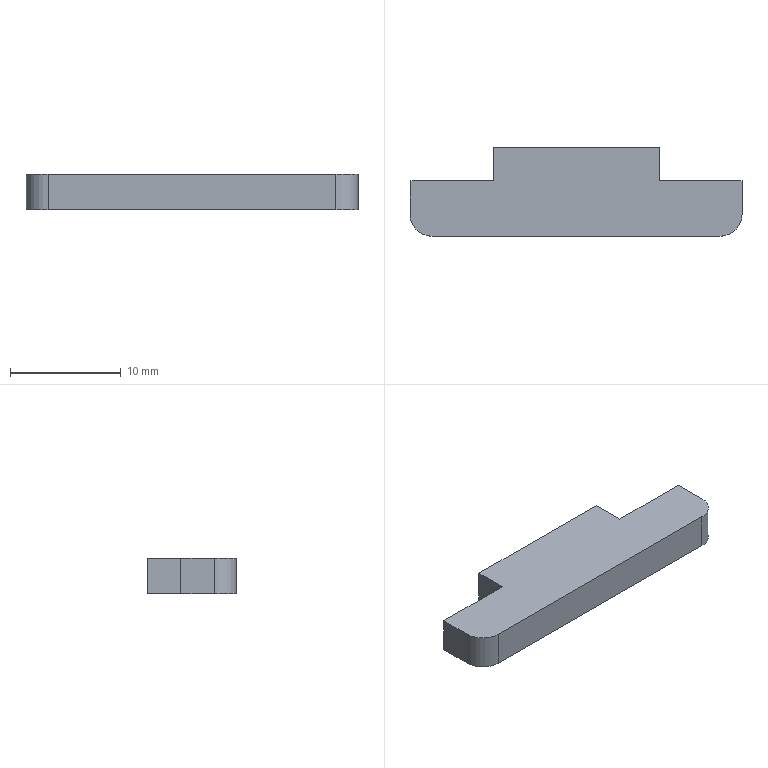Part | SolidWorks | features FlatPattern 1, SMBaseFlange 1, SheetMetal 1 | 1 solid | 12 faces | box 30 x 8 x 3.2 mm | volume 618.506 mm3 | plane 10 | cylinder 2 | commonest cylinder face diameters 4 x2
STEP:
#1=CARTESIAN_POINT('',(-119.188,177.146,0.));
#2=VERTEX_POINT('',#1);
#3=CARTESIAN_POINT('',(-119.188,180.146,0.));
#4=VERTEX_POINT('',#3);
#5=CARTESIAN_POINT('',(-119.188,177.146,0.));
#6=DIRECTION('',(0.,1.,0.));
#7=VECTOR('',#6,1000.);
#8=LINE('',#5,#7);
#9=EDGE_CURVE('',#2,#4,#8,.T.);
#10=ORIENTED_EDGE('',*,*,#9,.F.);
#11=CARTESIAN_POINT('',(-119.188,177.146,-3.2));
#12=VERTEX_POINT('',#11);
#13=CARTESIAN_POINT('',(-119.188,177.146,-3.2));
#14=DIRECTION('',(0.,0.,1.));
#15=VECTOR('',#14,1000.);
#16=LINE('',#13,#15);
#17=EDGE_CURVE('',#12,#2,#16,.T.);
#18=ORIENTED_EDGE('',*,*,#17,.F.);
#19=CARTESIAN_POINT('',(-119.188,180.146,-3.2));
#20=VERTEX_POINT('',#19);
#21=CARTESIAN_POINT('',(-119.188,177.146,-3.2));
#22=DIRECTION('',(0.,1.,0.));
#23=VECTOR('',#22,1000.);
#24=LINE('',#21,#23);
#25=EDGE_CURVE('',#12,#20,#24,.T.);
#26=ORIENTED_EDGE('',*,*,#25,.T.);
#27=CARTESIAN_POINT('',(-119.188,180.146,-3.2));
#28=DIRECTION('',(0.,0.,1.));
#29=VECTOR('',#28,1000.);
#30=LINE('',#27,#29);
#31=EDGE_CURVE('',#20,#4,#30,.T.);
#32=ORIENTED_EDGE('',*,*,#31,.T.);
#33=EDGE_LOOP('',(#10,#18,#26,#32));
#34=FACE_OUTER_BOUND('',#33,.T.);
#35=CARTESIAN_POINT('',(-119.188,177.146,-3.2));
#36=DIRECTION('',(1.,0.,0.));
#37=DIRECTION('',(0.,0.,-1.));
#38=AXIS2_PLACEMENT_3D('',#35,#36,#37);
#39=PLANE('',#38);
#40=ADVANCED_FACE('',(#34),#39,.T.);
#41=CARTESIAN_POINT('',(-121.188,175.146,0.));
#42=VERTEX_POINT('',#41);
#43=CARTESIAN_POINT('',(-121.188,177.146,0.));
#44=DIRECTION('',(0.,0.,1.));
#45=DIRECTION('',(1.,0.,0.));
#46=AXIS2_PLACEMENT_3D('',#43,#44,#45);
#47=CIRCLE('',#46,2.);
#48=EDGE_CURVE('',#42,#2,#47,.T.);
#49=ORIENTED_EDGE('',*,*,#48,.F.);
#50=CARTESIAN_POINT('',(-121.188,175.146,-3.2));
#51=VERTEX_POINT('',#50);
#52=CARTESIAN_POINT('',(-121.188,175.146,-3.2));
#53=DIRECTION('',(0.,0.,1.));
#54=VECTOR('',#53,1000.);
#55=LINE('',#52,#54);
#56=EDGE_CURVE('',#51,#42,#55,.T.);
#57=ORIENTED_EDGE('',*,*,#56,.F.);
#58=CARTESIAN_POINT('',(-121.188,177.146,-3.2));
#59=DIRECTION('',(0.,0.,1.));
#60=DIRECTION('',(1.,0.,0.));
#61=AXIS2_PLACEMENT_3D('',#58,#59,#60);
#62=CIRCLE('',#61,2.);
#63=EDGE_CURVE('',#51,#12,#62,.T.);
#64=ORIENTED_EDGE('',*,*,#63,.T.);
#65=ORIENTED_EDGE('',*,*,#17,.T.);
#66=EDGE_LOOP('',(#49,#57,#64,#65));
#67=FACE_OUTER_BOUND('',#66,.T.);
#68=CARTESIAN_POINT('',(-121.188,177.146,-3.2));
#69=DIRECTION('',(0.,0.,1.));
#70=DIRECTION('',(1.,0.,0.));
#71=AXIS2_PLACEMENT_3D('',#68,#69,#70);
#72=CYLINDRICAL_SURFACE('',#71,2.);
#73=ADVANCED_FACE('',(#67),#72,.T.);
#74=CARTESIAN_POINT('',(-147.188,175.146,0.));
#75=VERTEX_POINT('',#74);
#76=CARTESIAN_POINT('',(-147.188,175.146,0.));
#77=DIRECTION('',(1.,0.,0.));
#78=VECTOR('',#77,1000.);
#79=LINE('',#76,#78);
#80=EDGE_CURVE('',#75,#42,#79,.T.);
#81=ORIENTED_EDGE('',*,*,#80,.F.);
#82=CARTESIAN_POINT('',(-147.188,175.146,-3.2));
#83=VERTEX_POINT('',#82);
#84=CARTESIAN_POINT('',(-147.188,175.146,-3.2));
#85=DIRECTION('',(0.,0.,1.));
#86=VECTOR('',#85,1000.);
#87=LINE('',#84,#86);
#88=EDGE_CURVE('',#83,#75,#87,.T.);
#89=ORIENTED_EDGE('',*,*,#88,.F.);
#90=CARTESIAN_POINT('',(-147.188,175.146,-3.2));
#91=DIRECTION('',(1.,0.,0.));
#92=VECTOR('',#91,1000.);
#93=LINE('',#90,#92);
#94=EDGE_CURVE('',#83,#51,#93,.T.);
#95=ORIENTED_EDGE('',*,*,#94,.T.);
#96=ORIENTED_EDGE('',*,*,#56,.T.);
#97=EDGE_LOOP('',(#81,#89,#95,#96));
#98=FACE_OUTER_BOUND('',#97,.T.);
#99=CARTESIAN_POINT('',(-147.188,175.146,-3.2));
#100=DIRECTION('',(0.,-1.,0.));
#101=DIRECTION('',(0.,0.,-1.));
#102=AXIS2_PLACEMENT_3D('',#99,#100,#101);
#103=PLANE('',#102);
#104=ADVANCED_FACE('',(#98),#103,.T.);
#105=CARTESIAN_POINT('',(-149.188,177.146,0.));
#106=VERTEX_POINT('',#105);
#107=CARTESIAN_POINT('',(-147.188,177.146,0.));
#108=DIRECTION('',(0.,0.,1.));
#109=DIRECTION('',(1.,0.,0.));
#110=AXIS2_PLACEMENT_3D('',#107,#108,#109);
#111=CIRCLE('',#110,2.);
#112=EDGE_CURVE('',#106,#75,#111,.T.);
#113=ORIENTED_EDGE('',*,*,#112,.F.);
#114=CARTESIAN_POINT('',(-149.188,177.146,-3.2));
#115=VERTEX_POINT('',#114);
#116=CARTESIAN_POINT('',(-149.188,177.146,-3.2));
#117=DIRECTION('',(0.,0.,1.));
#118=VECTOR('',#117,1000.);
#119=LINE('',#116,#118);
#120=EDGE_CURVE('',#115,#106,#119,.T.);
#121=ORIENTED_EDGE('',*,*,#120,.F.);
#122=CARTESIAN_POINT('',(-147.188,177.146,-3.2));
#123=DIRECTION('',(0.,0.,1.));
#124=DIRECTION('',(1.,0.,0.));
#125=AXIS2_PLACEMENT_3D('',#122,#123,#124);
#126=CIRCLE('',#125,2.);
#127=EDGE_CURVE('',#115,#83,#126,.T.);
#128=ORIENTED_EDGE('',*,*,#127,.T.);
#129=ORIENTED_EDGE('',*,*,#88,.T.);
#130=EDGE_LOOP('',(#113,#121,#128,#129));
#131=FACE_OUTER_BOUND('',#130,.T.);
#132=CARTESIAN_POINT('',(-147.188,177.146,-3.2));
#133=DIRECTION('',(0.,0.,1.));
#134=DIRECTION('',(1.,0.,0.));
#135=AXIS2_PLACEMENT_3D('',#132,#133,#134);
#136=CYLINDRICAL_SURFACE('',#135,2.);
#137=ADVANCED_FACE('',(#131),#136,.T.);
#138=CARTESIAN_POINT('',(-149.188,180.146,0.));
#139=VERTEX_POINT('',#138);
#140=CARTESIAN_POINT('',(-149.188,180.146,0.));
#141=DIRECTION('',(0.,-1.,0.));
#142=VECTOR('',#141,1000.);
#143=LINE('',#140,#142);
#144=EDGE_CURVE('',#139,#106,#143,.T.);
#145=ORIENTED_EDGE('',*,*,#144,.F.);
#146=CARTESIAN_POINT('',(-149.188,180.146,-3.2));
#147=VERTEX_POINT('',#146);
#148=CARTESIAN_POINT('',(-149.188,180.146,-3.2));
#149=DIRECTION('',(0.,0.,1.));
#150=VECTOR('',#149,1000.);
#151=LINE('',#148,#150);
#152=EDGE_CURVE('',#147,#139,#151,.T.);
#153=ORIENTED_EDGE('',*,*,#152,.F.);
#154=CARTESIAN_POINT('',(-149.188,180.146,-3.2));
#155=DIRECTION('',(0.,-1.,0.));
#156=VECTOR('',#155,1000.);
#157=LINE('',#154,#156);
#158=EDGE_CURVE('',#147,#115,#157,.T.);
#159=ORIENTED_EDGE('',*,*,#158,.T.);
#160=ORIENTED_EDGE('',*,*,#120,.T.);
#161=EDGE_LOOP('',(#145,#153,#159,#160));
#162=FACE_OUTER_BOUND('',#161,.T.);
#163=CARTESIAN_POINT('',(-149.188,180.146,-3.2));
#164=DIRECTION('',(-1.,0.,0.));
#165=DIRECTION('',(0.,0.,1.));
#166=AXIS2_PLACEMENT_3D('',#163,#164,#165);
#167=PLANE('',#166);
#168=ADVANCED_FACE('',(#162),#167,.T.);
#169=CARTESIAN_POINT('',(-141.688,180.146,0.));
#170=VERTEX_POINT('',#169);
#171=CARTESIAN_POINT('',(-141.688,180.146,0.));
#172=DIRECTION('',(-1.,0.,0.));
#173=VECTOR('',#172,1000.);
#174=LINE('',#171,#173);
#175=EDGE_CURVE('',#170,#139,#174,.T.);
#176=ORIENTED_EDGE('',*,*,#175,.F.);
#177=CARTESIAN_POINT('',(-141.688,180.146,-3.2));
#178=VERTEX_POINT('',#177);
#179=CARTESIAN_POINT('',(-141.688,180.146,-3.2));
#180=DIRECTION('',(0.,0.,1.));
#181=VECTOR('',#180,1000.);
#182=LINE('',#179,#181);
#183=EDGE_CURVE('',#178,#170,#182,.T.);
#184=ORIENTED_EDGE('',*,*,#183,.F.);
#185=CARTESIAN_POINT('',(-141.688,180.146,-3.2));
#186=DIRECTION('',(-1.,0.,0.));
#187=VECTOR('',#186,1000.);
#188=LINE('',#185,#187);
#189=EDGE_CURVE('',#178,#147,#188,.T.);
#190=ORIENTED_EDGE('',*,*,#189,.T.);
#191=ORIENTED_EDGE('',*,*,#152,.T.);
#192=EDGE_LOOP('',(#176,#184,#190,#191));
#193=FACE_OUTER_BOUND('',#192,.T.);
#194=CARTESIAN_POINT('',(-141.688,180.146,-3.2));
#195=DIRECTION('',(0.,1.,0.));
#196=DIRECTION('',(0.,0.,1.));
#197=AXIS2_PLACEMENT_3D('',#194,#195,#196);
#198=PLANE('',#197);
#199=ADVANCED_FACE('',(#193),#198,.T.);
#200=CARTESIAN_POINT('',(-141.688,183.146,0.));
#201=VERTEX_POINT('',#200);
#202=CARTESIAN_POINT('',(-141.688,183.146,0.));
#203=DIRECTION('',(0.,-1.,0.));
#204=VECTOR('',#203,1000.);
#205=LINE('',#202,#204);
#206=EDGE_CURVE('',#201,#170,#205,.T.);
#207=ORIENTED_EDGE('',*,*,#206,.F.);
#208=CARTESIAN_POINT('',(-141.688,183.146,-3.2));
#209=VERTEX_POINT('',#208);
#210=CARTESIAN_POINT('',(-141.688,183.146,-3.2));
#211=DIRECTION('',(0.,0.,1.));
#212=VECTOR('',#211,1000.);
#213=LINE('',#210,#212);
#214=EDGE_CURVE('',#209,#201,#213,.T.);
#215=ORIENTED_EDGE('',*,*,#214,.F.);
#216=CARTESIAN_POINT('',(-141.688,183.146,-3.2));
#217=DIRECTION('',(0.,-1.,0.));
#218=VECTOR('',#217,1000.);
#219=LINE('',#216,#218);
#220=EDGE_CURVE('',#209,#178,#219,.T.);
#221=ORIENTED_EDGE('',*,*,#220,.T.);
#222=ORIENTED_EDGE('',*,*,#183,.T.);
#223=EDGE_LOOP('',(#207,#215,#221,#222));
#224=FACE_OUTER_BOUND('',#223,.T.);
#225=CARTESIAN_POINT('',(-141.688,183.146,-3.2));
#226=DIRECTION('',(-1.,0.,0.));
#227=DIRECTION('',(0.,0.,1.));
#228=AXIS2_PLACEMENT_3D('',#225,#226,#227);
#229=PLANE('',#228);
#230=ADVANCED_FACE('',(#224),#229,.T.);
#231=CARTESIAN_POINT('',(-126.688,183.146,0.));
#232=VERTEX_POINT('',#231);
#233=CARTESIAN_POINT('',(-126.688,183.146,0.));
#234=DIRECTION('',(-1.,0.,0.));
#235=VECTOR('',#234,1000.);
#236=LINE('',#233,#235);
#237=EDGE_CURVE('',#232,#201,#236,.T.);
#238=ORIENTED_EDGE('',*,*,#237,.F.);
#239=CARTESIAN_POINT('',(-126.688,183.146,-3.2));
#240=VERTEX_POINT('',#239);
#241=CARTESIAN_POINT('',(-126.688,183.146,-3.2));
#242=DIRECTION('',(0.,0.,1.));
#243=VECTOR('',#242,1000.);
#244=LINE('',#241,#243);
#245=EDGE_CURVE('',#240,#232,#244,.T.);
#246=ORIENTED_EDGE('',*,*,#245,.F.);
#247=CARTESIAN_POINT('',(-126.688,183.146,-3.2));
#248=DIRECTION('',(-1.,0.,0.));
#249=VECTOR('',#248,1000.);
#250=LINE('',#247,#249);
#251=EDGE_CURVE('',#240,#209,#250,.T.);
#252=ORIENTED_EDGE('',*,*,#251,.T.);
#253=ORIENTED_EDGE('',*,*,#214,.T.);
#254=EDGE_LOOP('',(#238,#246,#252,#253));
#255=FACE_OUTER_BOUND('',#254,.T.);
#256=CARTESIAN_POINT('',(-126.688,183.146,-3.2));
#257=DIRECTION('',(0.,1.,0.));
#258=DIRECTION('',(0.,0.,1.));
#259=AXIS2_PLACEMENT_3D('',#256,#257,#258);
#260=PLANE('',#259);
#261=ADVANCED_FACE('',(#255),#260,.T.);
#262=CARTESIAN_POINT('',(-126.688,180.146,0.));
#263=VERTEX_POINT('',#262);
#264=CARTESIAN_POINT('',(-126.688,180.146,0.));
#265=DIRECTION('',(0.,1.,0.));
#266=VECTOR('',#265,1000.);
#267=LINE('',#264,#266);
#268=EDGE_CURVE('',#263,#232,#267,.T.);
#269=ORIENTED_EDGE('',*,*,#268,.F.);
#270=CARTESIAN_POINT('',(-126.688,180.146,-3.2));
#271=VERTEX_POINT('',#270);
#272=CARTESIAN_POINT('',(-126.688,180.146,-3.2));
#273=DIRECTION('',(0.,0.,1.));
#274=VECTOR('',#273,1000.);
#275=LINE('',#272,#274);
#276=EDGE_CURVE('',#271,#263,#275,.T.);
#277=ORIENTED_EDGE('',*,*,#276,.F.);
#278=CARTESIAN_POINT('',(-126.688,180.146,-3.2));
#279=DIRECTION('',(0.,1.,0.));
#280=VECTOR('',#279,1000.);
#281=LINE('',#278,#280);
#282=EDGE_CURVE('',#271,#240,#281,.T.);
#283=ORIENTED_EDGE('',*,*,#282,.T.);
#284=ORIENTED_EDGE('',*,*,#245,.T.);
#285=EDGE_LOOP('',(#269,#277,#283,#284));
#286=FACE_OUTER_BOUND('',#285,.T.);
#287=CARTESIAN_POINT('',(-126.688,180.146,-3.2));
#288=DIRECTION('',(1.,0.,0.));
#289=DIRECTION('',(0.,0.,-1.));
#290=AXIS2_PLACEMENT_3D('',#287,#288,#289);
#291=PLANE('',#290);
#292=ADVANCED_FACE('',(#286),#291,.T.);
#293=CARTESIAN_POINT('',(-119.188,180.146,0.));
#294=DIRECTION('',(-1.,0.,0.));
#295=VECTOR('',#294,1000.);
#296=LINE('',#293,#295);
#297=EDGE_CURVE('',#4,#263,#296,.T.);
#298=ORIENTED_EDGE('',*,*,#297,.F.);
#299=ORIENTED_EDGE('',*,*,#31,.F.);
#300=CARTESIAN_POINT('',(-119.188,180.146,-3.2));
#301=DIRECTION('',(-1.,0.,0.));
#302=VECTOR('',#301,1000.);
#303=LINE('',#300,#302);
#304=EDGE_CURVE('',#20,#271,#303,.T.);
#305=ORIENTED_EDGE('',*,*,#304,.T.);
#306=ORIENTED_EDGE('',*,*,#276,.T.);
#307=EDGE_LOOP('',(#298,#299,#305,#306));
#308=FACE_OUTER_BOUND('',#307,.T.);
#309=CARTESIAN_POINT('',(-119.188,180.146,-3.2));
#310=DIRECTION('',(0.,1.,0.));
#311=DIRECTION('',(0.,0.,1.));
#312=AXIS2_PLACEMENT_3D('',#309,#310,#311);
#313=PLANE('',#312);
#314=ADVANCED_FACE('',(#308),#313,.T.);
#315=ORIENTED_EDGE('',*,*,#25,.F.);
#316=ORIENTED_EDGE('',*,*,#63,.F.);
#317=ORIENTED_EDGE('',*,*,#94,.F.);
#318=ORIENTED_EDGE('',*,*,#127,.F.);
#319=ORIENTED_EDGE('',*,*,#158,.F.);
#320=ORIENTED_EDGE('',*,*,#189,.F.);
#321=ORIENTED_EDGE('',*,*,#220,.F.);
#322=ORIENTED_EDGE('',*,*,#251,.F.);
#323=ORIENTED_EDGE('',*,*,#282,.F.);
#324=ORIENTED_EDGE('',*,*,#304,.F.);
#325=EDGE_LOOP('',(#315,#316,#317,#318,#319,#320,#321,#322,#323,#324));
#326=FACE_OUTER_BOUND('',#325,.T.);
#327=CARTESIAN_POINT('',(-147.188,177.146,-3.2));
#328=DIRECTION('',(0.,0.,1.));
#329=DIRECTION('',(1.,0.,0.));
#330=AXIS2_PLACEMENT_3D('',#327,#328,#329);
#331=PLANE('',#330);
#332=ADVANCED_FACE('',(#326),#331,.F.);
#333=ORIENTED_EDGE('',*,*,#9,.T.);
#334=ORIENTED_EDGE('',*,*,#297,.T.);
#335=ORIENTED_EDGE('',*,*,#268,.T.);
#336=ORIENTED_EDGE('',*,*,#237,.T.);
#337=ORIENTED_EDGE('',*,*,#206,.T.);
#338=ORIENTED_EDGE('',*,*,#175,.T.);
#339=ORIENTED_EDGE('',*,*,#144,.T.);
#340=ORIENTED_EDGE('',*,*,#112,.T.);
#341=ORIENTED_EDGE('',*,*,#80,.T.);
#342=ORIENTED_EDGE('',*,*,#48,.T.);
#343=EDGE_LOOP('',(#333,#334,#335,#336,#337,#338,#339,#340,#341,#342));
#344=FACE_OUTER_BOUND('',#343,.T.);
#345=CARTESIAN_POINT('',(-147.188,177.146,0.));
#346=DIRECTION('',(0.,0.,1.));
#347=DIRECTION('',(1.,0.,0.));
#348=AXIS2_PLACEMENT_3D('',#345,#346,#347);
#349=PLANE('',#348);
#350=ADVANCED_FACE('',(#344),#349,.T.);
#351=CLOSED_SHELL('',(#40,#73,#104,#137,#168,#199,#230,#261,#292,#314,#332,#350));
#352=MANIFOLD_SOLID_BREP('',#351);
#353=CARTESIAN_POINT('',(0.,0.,0.));
#354=DIRECTION('',(0.,0.,1.));
#355=DIRECTION('',(1.,0.,0.));
#356=AXIS2_PLACEMENT_3D('',#353,#354,#355);
#357=(LENGTH_UNIT()NAMED_UNIT(*)SI_UNIT(.MILLI.,.METRE.));
#358=UNCERTAINTY_MEASURE_WITH_UNIT(LENGTH_MEASURE(0.00001),#357,'','');
#359=(NAMED_UNIT(*)PLANE_ANGLE_UNIT()SI_UNIT($,.RADIAN.));
#360=(NAMED_UNIT(*)SI_UNIT($,.STERADIAN.)SOLID_ANGLE_UNIT());
#361=(GEOMETRIC_REPRESENTATION_CONTEXT(3)GLOBAL_UNCERTAINTY_ASSIGNED_CONTEXT((#358))GLOBAL_UNIT_ASSIGNED_CONTEXT((#357,#359,#360))REPRESENTATION_CONTEXT('',''));
#362=ADVANCED_BREP_SHAPE_REPRESENTATION('',(#352,#356),#361);